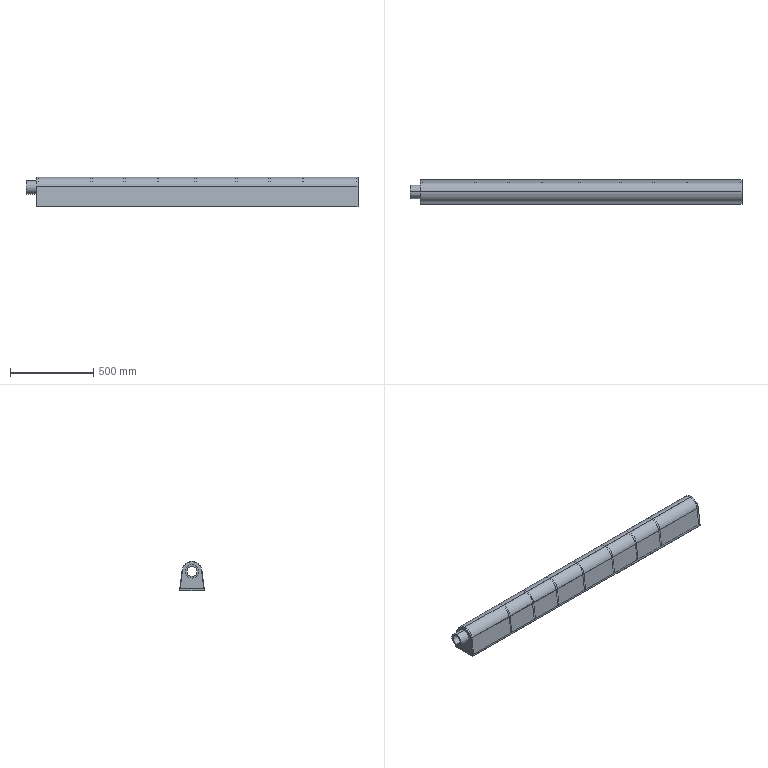Part | SolidWorks | features ICE 6, LPattern 3, Extrusion 1, MirrorSolid 1 | 13 solids | 106 faces | box 1995 x 150 x 175 mm | volume 11290061 mm3 | plane 67 | cylinder 39 | commonest cylinder face diameters 80 x20 116 x11 10 x4 60 x2 120 x2